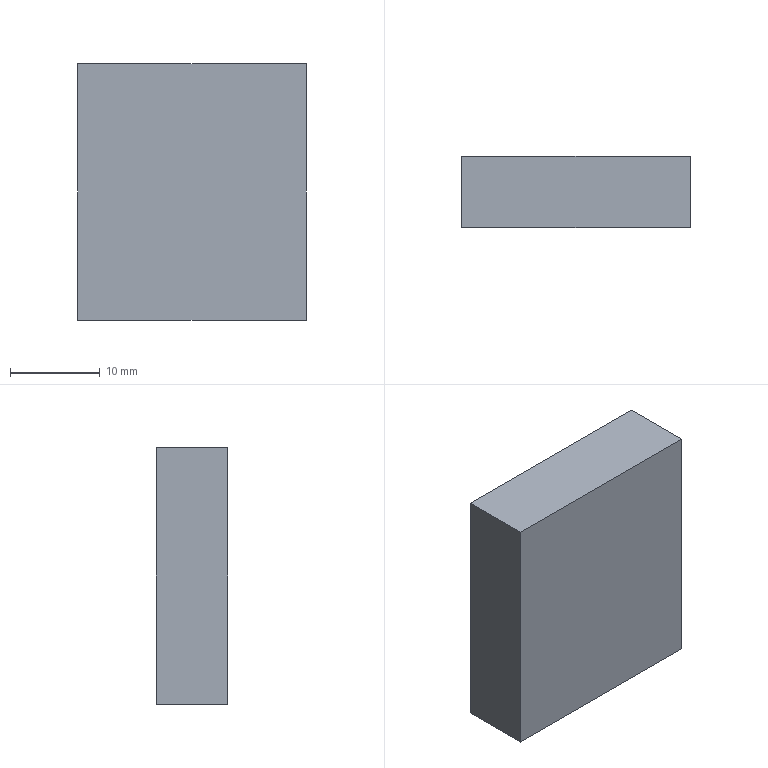Part | NX | features BREP 1 | 1 solid | 6 faces | box 25.4 x 7.938 x 28.575 mm | volume 5761 mm3 | plane 6
STEP:
#1=CARTESIAN_POINT('',(12.7,0.,-14.287));
#2=VERTEX_POINT('',#1);
#3=CARTESIAN_POINT('',(-12.7,0.,-14.287));
#4=VERTEX_POINT('',#3);
#5=CARTESIAN_POINT('',(12.7,0.,-14.287));
#6=DIRECTION('',(-1.,0.,0.));
#7=VECTOR('',#6,1000.);
#8=LINE('',#5,#7);
#9=EDGE_CURVE('',#2,#4,#8,.T.);
#10=ORIENTED_EDGE('',*,*,#9,.F.);
#11=CARTESIAN_POINT('',(12.7,0.,14.287));
#12=VERTEX_POINT('',#11);
#13=CARTESIAN_POINT('',(12.7,0.,14.287));
#14=DIRECTION('',(0.,0.,-1.));
#15=VECTOR('',#14,1000.);
#16=LINE('',#13,#15);
#17=EDGE_CURVE('',#12,#2,#16,.T.);
#18=ORIENTED_EDGE('',*,*,#17,.F.);
#19=CARTESIAN_POINT('',(-12.7,0.,14.287));
#20=VERTEX_POINT('',#19);
#21=CARTESIAN_POINT('',(-12.7,0.,14.287));
#22=DIRECTION('',(1.,0.,0.));
#23=VECTOR('',#22,1000.);
#24=LINE('',#21,#23);
#25=EDGE_CURVE('',#20,#12,#24,.T.);
#26=ORIENTED_EDGE('',*,*,#25,.F.);
#27=CARTESIAN_POINT('',(-12.7,0.,-14.287));
#28=DIRECTION('',(0.,0.,1.));
#29=VECTOR('',#28,1000.);
#30=LINE('',#27,#29);
#31=EDGE_CURVE('',#4,#20,#30,.T.);
#32=ORIENTED_EDGE('',*,*,#31,.F.);
#33=EDGE_LOOP('',(#10,#18,#26,#32));
#34=FACE_BOUND('',#33,.T.);
#35=CARTESIAN_POINT('',(0.,0.,0.));
#36=DIRECTION('',(0.,1.,0.));
#37=DIRECTION('',(1.,0.,0.));
#38=AXIS2_PLACEMENT_3D('',#35,#36,#37);
#39=PLANE('',#38);
#40=ADVANCED_FACE('',(#34),#39,.F.);
#41=CARTESIAN_POINT('',(-12.7,7.938,14.287));
#42=VERTEX_POINT('',#41);
#43=CARTESIAN_POINT('',(-12.7,0.,14.287));
#44=DIRECTION('',(0.,1.,0.));
#45=VECTOR('',#44,1000.);
#46=LINE('',#43,#45);
#47=EDGE_CURVE('',#20,#42,#46,.T.);
#48=ORIENTED_EDGE('',*,*,#47,.T.);
#49=CARTESIAN_POINT('',(-12.7,7.938,-14.287));
#50=VERTEX_POINT('',#49);
#51=CARTESIAN_POINT('',(-12.7,7.938,-14.287));
#52=DIRECTION('',(0.,0.,1.));
#53=VECTOR('',#52,1000.);
#54=LINE('',#51,#53);
#55=EDGE_CURVE('',#50,#42,#54,.T.);
#56=ORIENTED_EDGE('',*,*,#55,.F.);
#57=CARTESIAN_POINT('',(-12.7,0.,-14.287));
#58=DIRECTION('',(0.,1.,0.));
#59=VECTOR('',#58,1000.);
#60=LINE('',#57,#59);
#61=EDGE_CURVE('',#4,#50,#60,.T.);
#62=ORIENTED_EDGE('',*,*,#61,.F.);
#63=ORIENTED_EDGE('',*,*,#31,.T.);
#64=EDGE_LOOP('',(#48,#56,#62,#63));
#65=FACE_BOUND('',#64,.T.);
#66=CARTESIAN_POINT('',(-12.7,0.,-14.287));
#67=DIRECTION('',(-1.,0.,0.));
#68=DIRECTION('',(0.,0.,1.));
#69=AXIS2_PLACEMENT_3D('',#66,#67,#68);
#70=PLANE('',#69);
#71=ADVANCED_FACE('',(#65),#70,.T.);
#72=ORIENTED_EDGE('',*,*,#61,.T.);
#73=CARTESIAN_POINT('',(12.7,7.938,-14.287));
#74=VERTEX_POINT('',#73);
#75=CARTESIAN_POINT('',(12.7,7.938,-14.287));
#76=DIRECTION('',(-1.,0.,0.));
#77=VECTOR('',#76,1000.);
#78=LINE('',#75,#77);
#79=EDGE_CURVE('',#74,#50,#78,.T.);
#80=ORIENTED_EDGE('',*,*,#79,.F.);
#81=CARTESIAN_POINT('',(12.7,0.,-14.287));
#82=DIRECTION('',(0.,1.,0.));
#83=VECTOR('',#82,1000.);
#84=LINE('',#81,#83);
#85=EDGE_CURVE('',#2,#74,#84,.T.);
#86=ORIENTED_EDGE('',*,*,#85,.F.);
#87=ORIENTED_EDGE('',*,*,#9,.T.);
#88=EDGE_LOOP('',(#72,#80,#86,#87));
#89=FACE_BOUND('',#88,.T.);
#90=CARTESIAN_POINT('',(12.7,0.,-14.287));
#91=DIRECTION('',(0.,0.,-1.));
#92=DIRECTION('',(0.,-1.,0.));
#93=AXIS2_PLACEMENT_3D('',#90,#91,#92);
#94=PLANE('',#93);
#95=ADVANCED_FACE('',(#89),#94,.T.);
#96=ORIENTED_EDGE('',*,*,#85,.T.);
#97=CARTESIAN_POINT('',(12.7,7.938,14.287));
#98=VERTEX_POINT('',#97);
#99=CARTESIAN_POINT('',(12.7,7.938,14.287));
#100=DIRECTION('',(0.,0.,-1.));
#101=VECTOR('',#100,1000.);
#102=LINE('',#99,#101);
#103=EDGE_CURVE('',#98,#74,#102,.T.);
#104=ORIENTED_EDGE('',*,*,#103,.F.);
#105=CARTESIAN_POINT('',(12.7,0.,14.287));
#106=DIRECTION('',(0.,1.,0.));
#107=VECTOR('',#106,1000.);
#108=LINE('',#105,#107);
#109=EDGE_CURVE('',#12,#98,#108,.T.);
#110=ORIENTED_EDGE('',*,*,#109,.F.);
#111=ORIENTED_EDGE('',*,*,#17,.T.);
#112=EDGE_LOOP('',(#96,#104,#110,#111));
#113=FACE_BOUND('',#112,.T.);
#114=CARTESIAN_POINT('',(12.7,0.,14.287));
#115=DIRECTION('',(1.,0.,0.));
#116=DIRECTION('',(0.,1.,0.));
#117=AXIS2_PLACEMENT_3D('',#114,#115,#116);
#118=PLANE('',#117);
#119=ADVANCED_FACE('',(#113),#118,.T.);
#120=ORIENTED_EDGE('',*,*,#109,.T.);
#121=CARTESIAN_POINT('',(-12.7,7.938,14.287));
#122=DIRECTION('',(1.,0.,0.));
#123=VECTOR('',#122,1000.);
#124=LINE('',#121,#123);
#125=EDGE_CURVE('',#42,#98,#124,.T.);
#126=ORIENTED_EDGE('',*,*,#125,.F.);
#127=ORIENTED_EDGE('',*,*,#47,.F.);
#128=ORIENTED_EDGE('',*,*,#25,.T.);
#129=EDGE_LOOP('',(#120,#126,#127,#128));
#130=FACE_BOUND('',#129,.T.);
#131=CARTESIAN_POINT('',(-12.7,0.,14.287));
#132=DIRECTION('',(0.,0.,1.));
#133=DIRECTION('',(1.,0.,0.));
#134=AXIS2_PLACEMENT_3D('',#131,#132,#133);
#135=PLANE('',#134);
#136=ADVANCED_FACE('',(#130),#135,.T.);
#137=ORIENTED_EDGE('',*,*,#125,.T.);
#138=ORIENTED_EDGE('',*,*,#103,.T.);
#139=ORIENTED_EDGE('',*,*,#79,.T.);
#140=ORIENTED_EDGE('',*,*,#55,.T.);
#141=EDGE_LOOP('',(#137,#138,#139,#140));
#142=FACE_BOUND('',#141,.T.);
#143=CARTESIAN_POINT('',(0.,7.938,0.));
#144=DIRECTION('',(0.,1.,0.));
#145=DIRECTION('',(1.,0.,0.));
#146=AXIS2_PLACEMENT_3D('',#143,#144,#145);
#147=PLANE('',#146);
#148=ADVANCED_FACE('',(#142),#147,.T.);
#149=CLOSED_SHELL('',(#40,#71,#95,#119,#136,#148));
#150=MANIFOLD_SOLID_BREP('',#149);
#151=(LENGTH_UNIT()NAMED_UNIT(*)SI_UNIT(.MILLI.,.METRE.));
#152=UNCERTAINTY_MEASURE_WITH_UNIT(LENGTH_MEASURE(0.00001),#151,'','');
#153=(NAMED_UNIT(*)PLANE_ANGLE_UNIT()SI_UNIT($,.RADIAN.));
#154=(NAMED_UNIT(*)SI_UNIT($,.STERADIAN.)SOLID_ANGLE_UNIT());
#155=(GEOMETRIC_REPRESENTATION_CONTEXT(3)GLOBAL_UNCERTAINTY_ASSIGNED_CONTEXT((#152))GLOBAL_UNIT_ASSIGNED_CONTEXT((#151,#153,#154))REPRESENTATION_CONTEXT('',''));
#156=ADVANCED_BREP_SHAPE_REPRESENTATION('',(#150),#155);